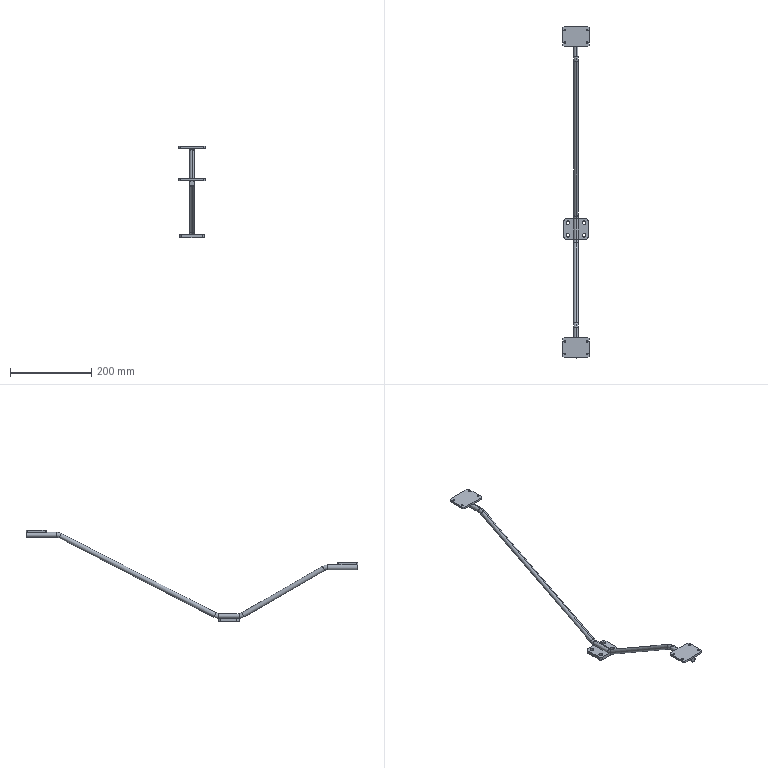Part | STEP file | HXGR200008-05-23 | 4 solids | 74 faces | box 65 x 818.205 x 225 mm | volume 155095 mm3 | cylinder 38 | plane 28 | torus 8 | commonest cylinder face diameters 4.2 x16 12 x10 9 x8 10 x4